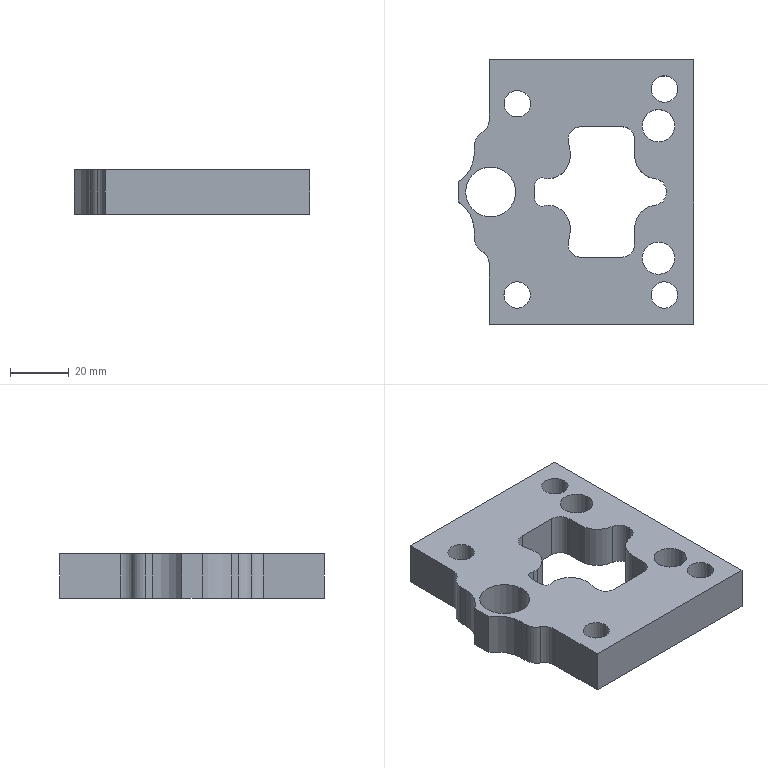Part | STEP file | 1 solid | 47 faces | box 80 x 90 x 15 mm | volume 69642 mm3 | cylinder 27 | plane 20 | commonest cylinder face diameters 8.28 x6 9 x4 10 x4 16.22 x4 5.28 x2 7.72 x2
STEP:
#1=CARTESIAN_POINT('',(347.5,22.5,-47.));
#2=VERTEX_POINT('',#1);
#3=CARTESIAN_POINT('',(342.,22.5,-47.));
#4=DIRECTION('',(0.,0.,1.));
#5=DIRECTION('',(1.,0.,0.));
#6=AXIS2_PLACEMENT_3D('',#3,#4,#5);
#7=CIRCLE('',#6,5.5);
#8=EDGE_CURVE('',#2,#2,#7,.T.);
#9=ORIENTED_EDGE('',*,*,#8,.T.);
#10=EDGE_LOOP('',(#9));
#11=FACE_BOUND('',#10,.T.);
#12=CARTESIAN_POINT('',(347.5,-22.5,-47.));
#13=VERTEX_POINT('',#12);
#14=CARTESIAN_POINT('',(342.,-22.5,-47.));
#15=DIRECTION('',(0.,0.,-1.));
#16=DIRECTION('',(1.,0.,0.));
#17=AXIS2_PLACEMENT_3D('',#14,#15,#16);
#18=CIRCLE('',#17,5.5);
#19=EDGE_CURVE('',#13,#13,#18,.T.);
#20=ORIENTED_EDGE('',*,*,#19,.F.);
#21=EDGE_LOOP('',(#20));
#22=FACE_BOUND('',#21,.T.);
#23=CARTESIAN_POINT('',(276.5,0.,-47.));
#24=VERTEX_POINT('',#23);
#25=CARTESIAN_POINT('',(285.,0.,-47.));
#26=DIRECTION('',(0.,0.,1.));
#27=DIRECTION('',(-1.,0.,0.));
#28=AXIS2_PLACEMENT_3D('',#25,#26,#27);
#29=CIRCLE('',#28,8.5);
#30=EDGE_CURVE('',#24,#24,#29,.T.);
#31=ORIENTED_EDGE('',*,*,#30,.T.);
#32=EDGE_LOOP('',(#31));
#33=FACE_BOUND('',#32,.T.);
#34=CARTESIAN_POINT('',(289.55,29.95,-47.));
#35=VERTEX_POINT('',#34);
#36=CARTESIAN_POINT('',(294.05,29.95,-47.));
#37=DIRECTION('',(0.,0.,1.));
#38=DIRECTION('',(-1.,0.,0.));
#39=AXIS2_PLACEMENT_3D('',#36,#37,#38);
#40=CIRCLE('',#39,4.5);
#41=EDGE_CURVE('',#35,#35,#40,.T.);
#42=ORIENTED_EDGE('',*,*,#41,.T.);
#43=EDGE_LOOP('',(#42));
#44=FACE_BOUND('',#43,.T.);
#45=CARTESIAN_POINT('',(339.55,34.95,-47.));
#46=VERTEX_POINT('',#45);
#47=CARTESIAN_POINT('',(344.05,34.95,-47.));
#48=DIRECTION('',(0.,0.,1.));
#49=DIRECTION('',(-1.,0.,0.));
#50=AXIS2_PLACEMENT_3D('',#47,#48,#49);
#51=CIRCLE('',#50,4.5);
#52=EDGE_CURVE('',#46,#46,#51,.T.);
#53=ORIENTED_EDGE('',*,*,#52,.T.);
#54=EDGE_LOOP('',(#53));
#55=FACE_BOUND('',#54,.T.);
#56=CARTESIAN_POINT('',(348.5,-35.,-47.));
#57=VERTEX_POINT('',#56);
#58=CARTESIAN_POINT('',(344.,-35.,-47.));
#59=DIRECTION('',(0.,0.,1.));
#60=DIRECTION('',(1.,0.,0.));
#61=AXIS2_PLACEMENT_3D('',#58,#59,#60);
#62=CIRCLE('',#61,4.5);
#63=EDGE_CURVE('',#57,#57,#62,.T.);
#64=ORIENTED_EDGE('',*,*,#63,.T.);
#65=EDGE_LOOP('',(#64));
#66=FACE_BOUND('',#65,.T.);
#67=CARTESIAN_POINT('',(298.5,-35.,-47.));
#68=VERTEX_POINT('',#67);
#69=CARTESIAN_POINT('',(294.,-35.,-47.));
#70=DIRECTION('',(0.,0.,1.));
#71=DIRECTION('',(1.,0.,0.));
#72=AXIS2_PLACEMENT_3D('',#69,#70,#71);
#73=CIRCLE('',#72,4.5);
#74=EDGE_CURVE('',#68,#68,#73,.T.);
#75=ORIENTED_EDGE('',*,*,#74,.T.);
#76=EDGE_LOOP('',(#75));
#77=FACE_BOUND('',#76,.T.);
#78=CARTESIAN_POINT('',(279.5,13.5,-47.));
#79=VERTEX_POINT('',#78);
#80=CARTESIAN_POINT('',(274.,3.413,-47.));
#81=VERTEX_POINT('',#80);
#82=CARTESIAN_POINT('',(267.5,13.5,-47.));
#83=DIRECTION('',(0.,0.,-1.));
#84=DIRECTION('',(-1.,0.,0.));
#85=AXIS2_PLACEMENT_3D('',#82,#83,#84);
#86=CIRCLE('',#85,12.);
#87=EDGE_CURVE('',#79,#81,#86,.T.);
#88=ORIENTED_EDGE('',*,*,#87,.F.);
#89=CARTESIAN_POINT('',(279.5,15.769,-47.));
#90=VERTEX_POINT('',#89);
#91=CARTESIAN_POINT('',(279.5,0.,-47.));
#92=DIRECTION('',(0.,-1.,0.));
#93=VECTOR('',#92,1.);
#94=LINE('',#91,#93);
#95=EDGE_CURVE('',#90,#79,#94,.T.);
#96=ORIENTED_EDGE('',*,*,#95,.F.);
#97=CARTESIAN_POINT('',(282.,20.099,-47.));
#98=VERTEX_POINT('',#97);
#99=CARTESIAN_POINT('',(284.5,15.769,-47.));
#100=DIRECTION('',(0.,0.,1.));
#101=DIRECTION('',(-1.,0.,0.));
#102=AXIS2_PLACEMENT_3D('',#99,#100,#101);
#103=CIRCLE('',#102,5.);
#104=EDGE_CURVE('',#98,#90,#103,.T.);
#105=ORIENTED_EDGE('',*,*,#104,.F.);
#106=CARTESIAN_POINT('',(284.5,24.429,-47.));
#107=VERTEX_POINT('',#106);
#108=CARTESIAN_POINT('',(279.5,24.429,-47.));
#109=DIRECTION('',(0.,0.,-1.));
#110=DIRECTION('',(-1.,0.,0.));
#111=AXIS2_PLACEMENT_3D('',#108,#109,#110);
#112=CIRCLE('',#111,5.);
#113=EDGE_CURVE('',#107,#98,#112,.T.);
#114=ORIENTED_EDGE('',*,*,#113,.F.);
#115=CARTESIAN_POINT('',(284.5,45.,-47.));
#116=VERTEX_POINT('',#115);
#117=CARTESIAN_POINT('',(284.5,0.,-47.));
#118=DIRECTION('',(0.,-1.,0.));
#119=VECTOR('',#118,1.);
#120=LINE('',#117,#119);
#121=EDGE_CURVE('',#116,#107,#120,.T.);
#122=ORIENTED_EDGE('',*,*,#121,.F.);
#123=CARTESIAN_POINT('',(354.,45.,-47.));
#124=VERTEX_POINT('',#123);
#125=CARTESIAN_POINT('',(323.,45.,-47.));
#126=DIRECTION('',(-1.,0.,0.));
#127=VECTOR('',#126,1.);
#128=LINE('',#125,#127);
#129=EDGE_CURVE('',#124,#116,#128,.T.);
#130=ORIENTED_EDGE('',*,*,#129,.F.);
#131=CARTESIAN_POINT('',(354.,-45.,-47.));
#132=VERTEX_POINT('',#131);
#133=CARTESIAN_POINT('',(354.,0.,-47.));
#134=DIRECTION('',(0.,1.,0.));
#135=VECTOR('',#134,1.);
#136=LINE('',#133,#135);
#137=EDGE_CURVE('',#132,#124,#136,.T.);
#138=ORIENTED_EDGE('',*,*,#137,.F.);
#139=CARTESIAN_POINT('',(284.5,-45.,-47.));
#140=VERTEX_POINT('',#139);
#141=CARTESIAN_POINT('',(323.,-45.,-47.));
#142=DIRECTION('',(1.,0.,0.));
#143=VECTOR('',#142,1.);
#144=LINE('',#141,#143);
#145=EDGE_CURVE('',#140,#132,#144,.T.);
#146=ORIENTED_EDGE('',*,*,#145,.F.);
#147=CARTESIAN_POINT('',(284.5,-24.429,-47.));
#148=VERTEX_POINT('',#147);
#149=CARTESIAN_POINT('',(284.5,0.,-47.));
#150=DIRECTION('',(0.,-1.,0.));
#151=VECTOR('',#150,1.);
#152=LINE('',#149,#151);
#153=EDGE_CURVE('',#148,#140,#152,.T.);
#154=ORIENTED_EDGE('',*,*,#153,.F.);
#155=CARTESIAN_POINT('',(282.,-20.099,-47.));
#156=VERTEX_POINT('',#155);
#157=CARTESIAN_POINT('',(279.5,-24.429,-47.));
#158=DIRECTION('',(0.,0.,1.));
#159=DIRECTION('',(-1.,0.,0.));
#160=AXIS2_PLACEMENT_3D('',#157,#158,#159);
#161=CIRCLE('',#160,5.);
#162=EDGE_CURVE('',#148,#156,#161,.T.);
#163=ORIENTED_EDGE('',*,*,#162,.T.);
#164=CARTESIAN_POINT('',(279.5,-15.769,-47.));
#165=VERTEX_POINT('',#164);
#166=CARTESIAN_POINT('',(284.5,-15.769,-47.));
#167=DIRECTION('',(0.,0.,-1.));
#168=DIRECTION('',(-1.,0.,0.));
#169=AXIS2_PLACEMENT_3D('',#166,#167,#168);
#170=CIRCLE('',#169,5.);
#171=EDGE_CURVE('',#156,#165,#170,.T.);
#172=ORIENTED_EDGE('',*,*,#171,.T.);
#173=CARTESIAN_POINT('',(279.5,-13.5,-47.));
#174=VERTEX_POINT('',#173);
#175=CARTESIAN_POINT('',(279.5,0.,-47.));
#176=DIRECTION('',(0.,-1.,0.));
#177=VECTOR('',#176,1.);
#178=LINE('',#175,#177);
#179=EDGE_CURVE('',#174,#165,#178,.T.);
#180=ORIENTED_EDGE('',*,*,#179,.F.);
#181=CARTESIAN_POINT('',(274.,-3.413,-47.));
#182=VERTEX_POINT('',#181);
#183=CARTESIAN_POINT('',(267.5,-13.5,-47.));
#184=DIRECTION('',(0.,0.,-1.));
#185=DIRECTION('',(-1.,0.,0.));
#186=AXIS2_PLACEMENT_3D('',#183,#184,#185);
#187=CIRCLE('',#186,12.);
#188=EDGE_CURVE('',#182,#174,#187,.T.);
#189=ORIENTED_EDGE('',*,*,#188,.F.);
#190=CARTESIAN_POINT('',(274.,0.,-47.));
#191=DIRECTION('',(0.,-1.,0.));
#192=VECTOR('',#191,1.);
#193=LINE('',#190,#192);
#194=EDGE_CURVE('',#81,#182,#193,.T.);
#195=ORIENTED_EDGE('',*,*,#194,.F.);
#196=EDGE_LOOP('',(#88,#96,#105,#114,#122,#130,#138,#146,#154,#163,#172,#180,#189,#195));
#197=FACE_BOUND('',#196,.T.);
#198=CARTESIAN_POINT('',(311.395,-17.285,-47.));
#199=VERTEX_POINT('',#198);
#200=CARTESIAN_POINT('',(315.473,-22.14,-47.));
#201=VERTEX_POINT('',#200);
#202=CARTESIAN_POINT('',(315.473,-18.,-47.));
#203=DIRECTION('',(0.,0.,1.));
#204=DIRECTION('',(-1.,0.,0.));
#205=AXIS2_PLACEMENT_3D('',#202,#203,#204);
#206=CIRCLE('',#205,4.14);
#207=EDGE_CURVE('',#199,#201,#206,.T.);
#208=ORIENTED_EDGE('',*,*,#207,.T.);
#209=CARTESIAN_POINT('',(329.75,-22.14,-47.));
#210=VERTEX_POINT('',#209);
#211=CARTESIAN_POINT('',(323.,-22.14,-47.));
#212=DIRECTION('',(-1.,0.,0.));
#213=VECTOR('',#212,1.);
#214=LINE('',#211,#213);
#215=EDGE_CURVE('',#210,#201,#214,.T.);
#216=ORIENTED_EDGE('',*,*,#215,.F.);
#217=CARTESIAN_POINT('',(333.89,-18.,-47.));
#218=VERTEX_POINT('',#217);
#219=CARTESIAN_POINT('',(329.75,-18.,-47.));
#220=DIRECTION('',(0.,0.,1.));
#221=DIRECTION('',(-1.,0.,0.));
#222=AXIS2_PLACEMENT_3D('',#219,#220,#221);
#223=CIRCLE('',#222,4.14);
#224=EDGE_CURVE('',#210,#218,#223,.T.);
#225=ORIENTED_EDGE('',*,*,#224,.T.);
#226=CARTESIAN_POINT('',(333.89,-12.5,-47.));
#227=VERTEX_POINT('',#226);
#228=CARTESIAN_POINT('',(333.89,0.,-47.));
#229=DIRECTION('',(0.,-1.,0.));
#230=VECTOR('',#229,1.);
#231=LINE('',#228,#230);
#232=EDGE_CURVE('',#227,#218,#231,.T.);
#233=ORIENTED_EDGE('',*,*,#232,.F.);
#234=CARTESIAN_POINT('',(341.007,-4.451,-47.));
#235=VERTEX_POINT('',#234);
#236=CARTESIAN_POINT('',(342.,-12.5,-47.));
#237=DIRECTION('',(0.,0.,1.));
#238=DIRECTION('',(-1.,0.,0.));
#239=AXIS2_PLACEMENT_3D('',#236,#237,#238);
#240=CIRCLE('',#239,8.11);
#241=EDGE_CURVE('',#235,#227,#240,.T.);
#242=ORIENTED_EDGE('',*,*,#241,.F.);
#243=CARTESIAN_POINT('',(344.64,-0.3422,-47.));
#244=VERTEX_POINT('',#243);
#245=CARTESIAN_POINT('',(340.5,-0.3422,-47.));
#246=DIRECTION('',(0.,0.,-1.));
#247=DIRECTION('',(-1.,0.,0.));
#248=AXIS2_PLACEMENT_3D('',#245,#246,#247);
#249=CIRCLE('',#248,4.14);
#250=EDGE_CURVE('',#244,#235,#249,.T.);
#251=ORIENTED_EDGE('',*,*,#250,.F.);
#252=CARTESIAN_POINT('',(344.64,0.3422,-47.));
#253=VERTEX_POINT('',#252);
#254=CARTESIAN_POINT('',(344.64,0.,-47.));
#255=DIRECTION('',(0.,-1.,0.));
#256=VECTOR('',#255,1.);
#257=LINE('',#254,#256);
#258=EDGE_CURVE('',#253,#244,#257,.T.);
#259=ORIENTED_EDGE('',*,*,#258,.F.);
#260=CARTESIAN_POINT('',(341.007,4.451,-47.));
#261=VERTEX_POINT('',#260);
#262=CARTESIAN_POINT('',(340.5,0.3422,-47.));
#263=DIRECTION('',(0.,0.,-1.));
#264=DIRECTION('',(-1.,0.,0.));
#265=AXIS2_PLACEMENT_3D('',#262,#263,#264);
#266=CIRCLE('',#265,4.14);
#267=EDGE_CURVE('',#261,#253,#266,.T.);
#268=ORIENTED_EDGE('',*,*,#267,.F.);
#269=CARTESIAN_POINT('',(333.89,12.5,-47.));
#270=VERTEX_POINT('',#269);
#271=CARTESIAN_POINT('',(342.,12.5,-47.));
#272=DIRECTION('',(0.,0.,1.));
#273=DIRECTION('',(-1.,0.,0.));
#274=AXIS2_PLACEMENT_3D('',#271,#272,#273);
#275=CIRCLE('',#274,8.11);
#276=EDGE_CURVE('',#270,#261,#275,.T.);
#277=ORIENTED_EDGE('',*,*,#276,.F.);
#278=CARTESIAN_POINT('',(333.89,18.,-47.));
#279=VERTEX_POINT('',#278);
#280=CARTESIAN_POINT('',(333.89,0.,-47.));
#281=DIRECTION('',(0.,-1.,0.));
#282=VECTOR('',#281,1.);
#283=LINE('',#280,#282);
#284=EDGE_CURVE('',#279,#270,#283,.T.);
#285=ORIENTED_EDGE('',*,*,#284,.F.);
#286=CARTESIAN_POINT('',(329.75,22.14,-47.));
#287=VERTEX_POINT('',#286);
#288=CARTESIAN_POINT('',(329.75,18.,-47.));
#289=DIRECTION('',(0.,0.,1.));
#290=DIRECTION('',(-1.,0.,0.));
#291=AXIS2_PLACEMENT_3D('',#288,#289,#290);
#292=CIRCLE('',#291,4.14);
#293=EDGE_CURVE('',#279,#287,#292,.T.);
#294=ORIENTED_EDGE('',*,*,#293,.T.);
#295=CARTESIAN_POINT('',(315.473,22.14,-47.));
#296=VERTEX_POINT('',#295);
#297=CARTESIAN_POINT('',(323.,22.14,-47.));
#298=DIRECTION('',(1.,0.,0.));
#299=VECTOR('',#298,1.);
#300=LINE('',#297,#299);
#301=EDGE_CURVE('',#296,#287,#300,.T.);
#302=ORIENTED_EDGE('',*,*,#301,.F.);
#303=CARTESIAN_POINT('',(311.395,17.285,-47.));
#304=VERTEX_POINT('',#303);
#305=CARTESIAN_POINT('',(315.473,18.,-47.));
#306=DIRECTION('',(0.,0.,1.));
#307=DIRECTION('',(-1.,0.,0.));
#308=AXIS2_PLACEMENT_3D('',#305,#306,#307);
#309=CIRCLE('',#308,4.14);
#310=EDGE_CURVE('',#296,#304,#309,.T.);
#311=ORIENTED_EDGE('',*,*,#310,.T.);
#312=CARTESIAN_POINT('',(311.988,13.9,-47.));
#313=VERTEX_POINT('',#312);
#314=CARTESIAN_POINT('',(314.681,-1.458,-47.));
#315=DIRECTION('',(-0.1727,0.985,0.));
#316=VECTOR('',#315,1.);
#317=LINE('',#314,#316);
#318=EDGE_CURVE('',#313,#304,#317,.T.);
#319=ORIENTED_EDGE('',*,*,#318,.F.);
#320=CARTESIAN_POINT('',(305.14,4.471,-47.));
#321=VERTEX_POINT('',#320);
#322=CARTESIAN_POINT('',(304.,12.5,-47.));
#323=DIRECTION('',(0.,0.,1.));
#324=DIRECTION('',(-1.,0.,0.));
#325=AXIS2_PLACEMENT_3D('',#322,#323,#324);
#326=CIRCLE('',#325,8.11);
#327=EDGE_CURVE('',#321,#313,#326,.T.);
#328=ORIENTED_EDGE('',*,*,#327,.F.);
#329=CARTESIAN_POINT('',(305.14,4.471,-47.));
#330=VERTEX_POINT('',#329);
#331=CARTESIAN_POINT('',(305.14,0.,-47.));
#332=DIRECTION('',(0.,-1.,0.));
#333=VECTOR('',#332,1.);
#334=LINE('',#331,#333);
#335=EDGE_CURVE('',#330,#321,#334,.T.);
#336=ORIENTED_EDGE('',*,*,#335,.F.);
#337=CARTESIAN_POINT('',(303.367,4.652,-47.));
#338=VERTEX_POINT('',#337);
#339=CARTESIAN_POINT('',(304.635,8.298,-47.));
#340=DIRECTION('',(0.,0.,1.));
#341=DIRECTION('',(-1.,0.,0.));
#342=AXIS2_PLACEMENT_3D('',#339,#340,#341);
#343=CIRCLE('',#342,3.86);
#344=EDGE_CURVE('',#338,#330,#343,.T.);
#345=ORIENTED_EDGE('',*,*,#344,.F.);
#346=CARTESIAN_POINT('',(299.86,2.158,-47.));
#347=VERTEX_POINT('',#346);
#348=CARTESIAN_POINT('',(302.5,2.158,-47.));
#349=DIRECTION('',(0.,0.,-1.));
#350=DIRECTION('',(-1.,0.,0.));
#351=AXIS2_PLACEMENT_3D('',#348,#349,#350);
#352=CIRCLE('',#351,2.64);
#353=EDGE_CURVE('',#347,#338,#352,.T.);
#354=ORIENTED_EDGE('',*,*,#353,.F.);
#355=CARTESIAN_POINT('',(299.86,-2.158,-47.));
#356=VERTEX_POINT('',#355);
#357=CARTESIAN_POINT('',(299.86,0.,-47.));
#358=DIRECTION('',(0.,1.,0.));
#359=VECTOR('',#358,1.);
#360=LINE('',#357,#359);
#361=EDGE_CURVE('',#356,#347,#360,.T.);
#362=ORIENTED_EDGE('',*,*,#361,.F.);
#363=CARTESIAN_POINT('',(303.367,-4.652,-47.));
#364=VERTEX_POINT('',#363);
#365=CARTESIAN_POINT('',(302.5,-2.158,-47.));
#366=DIRECTION('',(0.,0.,-1.));
#367=DIRECTION('',(-1.,0.,0.));
#368=AXIS2_PLACEMENT_3D('',#365,#366,#367);
#369=CIRCLE('',#368,2.64);
#370=EDGE_CURVE('',#364,#356,#369,.T.);
#371=ORIENTED_EDGE('',*,*,#370,.F.);
#372=CARTESIAN_POINT('',(305.14,-4.471,-47.));
#373=VERTEX_POINT('',#372);
#374=CARTESIAN_POINT('',(304.635,-8.298,-47.));
#375=DIRECTION('',(0.,0.,1.));
#376=DIRECTION('',(-1.,0.,0.));
#377=AXIS2_PLACEMENT_3D('',#374,#375,#376);
#378=CIRCLE('',#377,3.86);
#379=EDGE_CURVE('',#373,#364,#378,.T.);
#380=ORIENTED_EDGE('',*,*,#379,.F.);
#381=CARTESIAN_POINT('',(305.14,-4.471,-47.));
#382=VERTEX_POINT('',#381);
#383=CARTESIAN_POINT('',(305.14,0.,-47.));
#384=DIRECTION('',(0.,-1.,0.));
#385=VECTOR('',#384,1.);
#386=LINE('',#383,#385);
#387=EDGE_CURVE('',#382,#373,#386,.T.);
#388=ORIENTED_EDGE('',*,*,#387,.F.);
#389=CARTESIAN_POINT('',(311.988,-13.9,-47.));
#390=VERTEX_POINT('',#389);
#391=CARTESIAN_POINT('',(304.,-12.5,-47.));
#392=DIRECTION('',(0.,0.,1.));
#393=DIRECTION('',(-1.,0.,0.));
#394=AXIS2_PLACEMENT_3D('',#391,#392,#393);
#395=CIRCLE('',#394,8.11);
#396=EDGE_CURVE('',#390,#382,#395,.T.);
#397=ORIENTED_EDGE('',*,*,#396,.F.);
#398=CARTESIAN_POINT('',(314.681,1.458,-47.));
#399=DIRECTION('',(0.1727,0.985,0.));
#400=VECTOR('',#399,1.);
#401=LINE('',#398,#400);
#402=EDGE_CURVE('',#199,#390,#401,.T.);
#403=ORIENTED_EDGE('',*,*,#402,.F.);
#404=EDGE_LOOP('',(#208,#216,#225,#233,#242,#251,#259,#268,#277,#285,#294,#302,#311,#319,#328,#336,#345,#354,#362,#371,#380,#388,#397,#403));
#405=FACE_BOUND('',#404,.T.);
#406=CARTESIAN_POINT('',(323.,0.,-47.));
#407=DIRECTION('',(0.,0.,-1.));
#408=DIRECTION('',(-1.,0.,0.));
#409=AXIS2_PLACEMENT_3D('',#406,#407,#408);
#410=PLANE('',#409);
#411=ADVANCED_FACE('',(#11,#22,#33,#44,#55,#66,#77,#197,#405),#410,.T.);
#412=CARTESIAN_POINT('',(274.,3.413,-32.));
#413=VERTEX_POINT('',#412);
#414=CARTESIAN_POINT('',(274.,-3.413,-32.));
#415=VERTEX_POINT('',#414);
#416=CARTESIAN_POINT('',(274.,0.,-32.));
#417=DIRECTION('',(0.,-1.,0.));
#418=VECTOR('',#417,1.);
#419=LINE('',#416,#418);
#420=EDGE_CURVE('',#413,#415,#419,.T.);
#421=ORIENTED_EDGE('',*,*,#420,.F.);
#422=CARTESIAN_POINT('',(274.,3.413,-53.));
#423=DIRECTION('',(0.,0.,-1.));
#424=VECTOR('',#423,1.);
#425=LINE('',#422,#424);
#426=EDGE_CURVE('',#413,#81,#425,.T.);
#427=ORIENTED_EDGE('',*,*,#426,.T.);
#428=ORIENTED_EDGE('',*,*,#194,.T.);
#429=CARTESIAN_POINT('',(274.,-3.413,-83.));
#430=DIRECTION('',(0.,0.,1.));
#431=VECTOR('',#430,1.);
#432=LINE('',#429,#431);
#433=EDGE_CURVE('',#182,#415,#432,.T.);
#434=ORIENTED_EDGE('',*,*,#433,.T.);
#435=EDGE_LOOP('',(#421,#427,#428,#434));
#436=FACE_OUTER_BOUND('',#435,.T.);
#437=CARTESIAN_POINT('',(274.,0.,-17.));
#438=DIRECTION('',(1.,0.,0.));
#439=DIRECTION('',(0.,0.,-1.));
#440=AXIS2_PLACEMENT_3D('',#437,#438,#439);
#441=PLANE('',#440);
#442=ADVANCED_FACE('',(#436),#441,.F.);
#443=ORIENTED_EDGE('',*,*,#129,.T.);
#444=CARTESIAN_POINT('',(284.5,45.,-32.));
#445=VERTEX_POINT('',#444);
#446=CARTESIAN_POINT('',(284.5,45.,-53.));
#447=DIRECTION('',(0.,0.,1.));
#448=VECTOR('',#447,1.);
#449=LINE('',#446,#448);
#450=EDGE_CURVE('',#116,#445,#449,.T.);
#451=ORIENTED_EDGE('',*,*,#450,.T.);
#452=CARTESIAN_POINT('',(354.,45.,-32.));
#453=VERTEX_POINT('',#452);
#454=CARTESIAN_POINT('',(323.,45.,-32.));
#455=DIRECTION('',(-1.,0.,0.));
#456=VECTOR('',#455,1.);
#457=LINE('',#454,#456);
#458=EDGE_CURVE('',#453,#445,#457,.T.);
#459=ORIENTED_EDGE('',*,*,#458,.F.);
#460=CARTESIAN_POINT('',(354.,45.,-32.));
#461=DIRECTION('',(0.,0.,-1.));
#462=VECTOR('',#461,1.);
#463=LINE('',#460,#462);
#464=EDGE_CURVE('',#453,#124,#463,.T.);
#465=ORIENTED_EDGE('',*,*,#464,.T.);
#466=EDGE_LOOP('',(#443,#451,#459,#465));
#467=FACE_OUTER_BOUND('',#466,.T.);
#468=CARTESIAN_POINT('',(323.,45.,-32.));
#469=DIRECTION('',(0.,-1.,0.));
#470=DIRECTION('',(-1.,0.,0.));
#471=AXIS2_PLACEMENT_3D('',#468,#469,#470);
#472=PLANE('',#471);
#473=ADVANCED_FACE('',(#467),#472,.F.);
#474=CARTESIAN_POINT('',(329.75,-22.14,-32.));
#475=VERTEX_POINT('',#474);
#476=CARTESIAN_POINT('',(315.473,-22.14,-32.));
#477=VERTEX_POINT('',#476);
#478=CARTESIAN_POINT('',(323.,-22.14,-32.));
#479=DIRECTION('',(-1.,0.,0.));
#480=VECTOR('',#479,1.);
#481=LINE('',#478,#480);
#482=EDGE_CURVE('',#475,#477,#481,.T.);
#483=ORIENTED_EDGE('',*,*,#482,.F.);
#484=CARTESIAN_POINT('',(329.75,-22.14,-32.));
#485=DIRECTION('',(0.,0.,-1.));
#486=VECTOR('',#485,1.);
#487=LINE('',#484,#486);
#488=EDGE_CURVE('',#475,#210,#487,.T.);
#489=ORIENTED_EDGE('',*,*,#488,.T.);
#490=ORIENTED_EDGE('',*,*,#215,.T.);
#491=CARTESIAN_POINT('',(315.473,-22.14,-32.));
#492=DIRECTION('',(0.,0.,-1.));
#493=VECTOR('',#492,1.);
#494=LINE('',#491,#493);
#495=EDGE_CURVE('',#477,#201,#494,.T.);
#496=ORIENTED_EDGE('',*,*,#495,.F.);
#497=EDGE_LOOP('',(#483,#489,#490,#496));
#498=FACE_OUTER_BOUND('',#497,.T.);
#499=CARTESIAN_POINT('',(323.,-22.14,-32.));
#500=DIRECTION('',(0.,-1.,0.));
#501=DIRECTION('',(-1.,0.,0.));
#502=AXIS2_PLACEMENT_3D('',#499,#500,#501);
#503=PLANE('',#502);
#504=ADVANCED_FACE('',(#498),#503,.F.);
#505=ORIENTED_EDGE('',*,*,#488,.F.);
#506=CARTESIAN_POINT('',(333.89,-18.,-32.));
#507=VERTEX_POINT('',#506);
#508=CARTESIAN_POINT('',(329.75,-18.,-32.));
#509=DIRECTION('',(0.,0.,1.));
#510=DIRECTION('',(-1.,0.,0.));
#511=AXIS2_PLACEMENT_3D('',#508,#509,#510);
#512=CIRCLE('',#511,4.14);
#513=EDGE_CURVE('',#475,#507,#512,.T.);
#514=ORIENTED_EDGE('',*,*,#513,.T.);
#515=CARTESIAN_POINT('',(333.89,-18.,-32.));
#516=DIRECTION('',(0.,0.,-1.));
#517=VECTOR('',#516,1.);
#518=LINE('',#515,#517);
#519=EDGE_CURVE('',#507,#218,#518,.T.);
#520=ORIENTED_EDGE('',*,*,#519,.T.);
#521=ORIENTED_EDGE('',*,*,#224,.F.);
#522=EDGE_LOOP('',(#505,#514,#520,#521));
#523=FACE_OUTER_BOUND('',#522,.T.);
#524=CARTESIAN_POINT('',(329.75,-18.,-32.));
#525=DIRECTION('',(0.,0.,-1.));
#526=DIRECTION('',(-1.,0.,0.));
#527=AXIS2_PLACEMENT_3D('',#524,#525,#526);
#528=CYLINDRICAL_SURFACE('',#527,4.14);
#529=ADVANCED_FACE('',(#523),#528,.F.);
#530=ORIENTED_EDGE('',*,*,#519,.F.);
#531=CARTESIAN_POINT('',(333.89,-12.5,-32.));
#532=VERTEX_POINT('',#531);
#533=CARTESIAN_POINT('',(333.89,0.,-32.));
#534=DIRECTION('',(0.,-1.,0.));
#535=VECTOR('',#534,1.);
#536=LINE('',#533,#535);
#537=EDGE_CURVE('',#532,#507,#536,.T.);
#538=ORIENTED_EDGE('',*,*,#537,.F.);
#539=CARTESIAN_POINT('',(333.89,-12.5,-32.));
#540=DIRECTION('',(0.,0.,-1.));
#541=VECTOR('',#540,1.);
#542=LINE('',#539,#541);
#543=EDGE_CURVE('',#532,#227,#542,.T.);
#544=ORIENTED_EDGE('',*,*,#543,.T.);
#545=ORIENTED_EDGE('',*,*,#232,.T.);
#546=EDGE_LOOP('',(#530,#538,#544,#545));
#547=FACE_OUTER_BOUND('',#546,.T.);
#548=CARTESIAN_POINT('',(333.89,0.,-32.));
#549=DIRECTION('',(-1.,0.,0.));
#550=DIRECTION('',(0.,1.,0.));
#551=AXIS2_PLACEMENT_3D('',#548,#549,#550);
#552=PLANE('',#551);
#553=ADVANCED_FACE('',(#547),#552,.T.);
#554=ORIENTED_EDGE('',*,*,#543,.F.);
#555=CARTESIAN_POINT('',(341.007,-4.451,-32.));
#556=VERTEX_POINT('',#555);
#557=CARTESIAN_POINT('',(342.,-12.5,-32.));
#558=DIRECTION('',(0.,0.,1.));
#559=DIRECTION('',(-1.,0.,0.));
#560=AXIS2_PLACEMENT_3D('',#557,#558,#559);
#561=CIRCLE('',#560,8.11);
#562=EDGE_CURVE('',#556,#532,#561,.T.);
#563=ORIENTED_EDGE('',*,*,#562,.F.);
#564=CARTESIAN_POINT('',(341.007,-4.451,-32.));
#565=DIRECTION('',(0.,0.,-1.));
#566=VECTOR('',#565,1.);
#567=LINE('',#564,#566);
#568=EDGE_CURVE('',#556,#235,#567,.T.);
#569=ORIENTED_EDGE('',*,*,#568,.T.);
#570=ORIENTED_EDGE('',*,*,#241,.T.);
#571=EDGE_LOOP('',(#554,#563,#569,#570));
#572=FACE_OUTER_BOUND('',#571,.T.);
#573=CARTESIAN_POINT('',(342.,-12.5,-32.));
#574=DIRECTION('',(0.,0.,-1.));
#575=DIRECTION('',(-1.,0.,0.));
#576=AXIS2_PLACEMENT_3D('',#573,#574,#575);
#577=CYLINDRICAL_SURFACE('',#576,8.11);
#578=ADVANCED_FACE('',(#572),#577,.T.);
#579=ORIENTED_EDGE('',*,*,#568,.F.);
#580=CARTESIAN_POINT('',(344.64,-0.3422,-32.));
#581=VERTEX_POINT('',#580);
#582=CARTESIAN_POINT('',(340.5,-0.3422,-32.));
#583=DIRECTION('',(0.,0.,-1.));
#584=DIRECTION('',(-1.,0.,0.));
#585=AXIS2_PLACEMENT_3D('',#582,#583,#584);
#586=CIRCLE('',#585,4.14);
#587=EDGE_CURVE('',#581,#556,#586,.T.);
#588=ORIENTED_EDGE('',*,*,#587,.F.);
#589=CARTESIAN_POINT('',(344.64,-0.3422,-32.));
#590=DIRECTION('',(0.,0.,-1.));
#591=VECTOR('',#590,1.);
#592=LINE('',#589,#591);
#593=EDGE_CURVE('',#581,#244,#592,.T.);
#594=ORIENTED_EDGE('',*,*,#593,.T.);
#595=ORIENTED_EDGE('',*,*,#250,.T.);
#596=EDGE_LOOP('',(#579,#588,#594,#595));
#597=FACE_OUTER_BOUND('',#596,.T.);
#598=CARTESIAN_POINT('',(340.5,-0.3422,-32.));
#599=DIRECTION('',(0.,0.,-1.));
#600=DIRECTION('',(-1.,0.,0.));
#601=AXIS2_PLACEMENT_3D('',#598,#599,#600);
#602=CYLINDRICAL_SURFACE('',#601,4.14);
#603=ADVANCED_FACE('',(#597),#602,.F.);
#604=ORIENTED_EDGE('',*,*,#593,.F.);
#605=CARTESIAN_POINT('',(344.64,0.3422,-32.));
#606=VERTEX_POINT('',#605);
#607=CARTESIAN_POINT('',(344.64,0.,-32.));
#608=DIRECTION('',(0.,-1.,0.));
#609=VECTOR('',#608,1.);
#610=LINE('',#607,#609);
#611=EDGE_CURVE('',#606,#581,#610,.T.);
#612=ORIENTED_EDGE('',*,*,#611,.F.);
#613=CARTESIAN_POINT('',(344.64,0.3422,-32.));
#614=DIRECTION('',(0.,0.,-1.));
#615=VECTOR('',#614,1.);
#616=LINE('',#613,#615);
#617=EDGE_CURVE('',#606,#253,#616,.T.);
#618=ORIENTED_EDGE('',*,*,#617,.T.);
#619=ORIENTED_EDGE('',*,*,#258,.T.);
#620=EDGE_LOOP('',(#604,#612,#618,#619));
#621=FACE_OUTER_BOUND('',#620,.T.);
#622=CARTESIAN_POINT('',(344.64,0.,-32.));
#623=DIRECTION('',(-1.,0.,0.));
#624=DIRECTION('',(0.,1.,0.));
#625=AXIS2_PLACEMENT_3D('',#622,#623,#624);
#626=PLANE('',#625);
#627=ADVANCED_FACE('',(#621),#626,.T.);
#628=ORIENTED_EDGE('',*,*,#617,.F.);
#629=CARTESIAN_POINT('',(341.007,4.451,-32.));
#630=VERTEX_POINT('',#629);
#631=CARTESIAN_POINT('',(340.5,0.3422,-32.));
#632=DIRECTION('',(0.,0.,-1.));
#633=DIRECTION('',(-1.,0.,0.));
#634=AXIS2_PLACEMENT_3D('',#631,#632,#633);
#635=CIRCLE('',#634,4.14);
#636=EDGE_CURVE('',#630,#606,#635,.T.);
#637=ORIENTED_EDGE('',*,*,#636,.F.);
#638=CARTESIAN_POINT('',(341.007,4.451,-32.));
#639=DIRECTION('',(0.,0.,-1.));
#640=VECTOR('',#639,1.);
#641=LINE('',#638,#640);
#642=EDGE_CURVE('',#630,#261,#641,.T.);
#643=ORIENTED_EDGE('',*,*,#642,.T.);
#644=ORIENTED_EDGE('',*,*,#267,.T.);
#645=EDGE_LOOP('',(#628,#637,#643,#644));
#646=FACE_OUTER_BOUND('',#645,.T.);
#647=CARTESIAN_POINT('',(340.5,0.3422,-32.));
#648=DIRECTION('',(0.,0.,-1.));
#649=DIRECTION('',(-1.,0.,0.));
#650=AXIS2_PLACEMENT_3D('',#647,#648,#649);
#651=CYLINDRICAL_SURFACE('',#650,4.14);
#652=ADVANCED_FACE('',(#646),#651,.F.);
#653=ORIENTED_EDGE('',*,*,#642,.F.);
#654=CARTESIAN_POINT('',(333.89,12.5,-32.));
#655=VERTEX_POINT('',#654);
#656=CARTESIAN_POINT('',(342.,12.5,-32.));
#657=DIRECTION('',(0.,0.,1.));
#658=DIRECTION('',(-1.,0.,0.));
#659=AXIS2_PLACEMENT_3D('',#656,#657,#658);
#660=CIRCLE('',#659,8.11);
#661=EDGE_CURVE('',#655,#630,#660,.T.);
#662=ORIENTED_EDGE('',*,*,#661,.F.);
#663=CARTESIAN_POINT('',(333.89,12.5,-32.));
#664=DIRECTION('',(0.,0.,-1.));
#665=VECTOR('',#664,1.);
#666=LINE('',#663,#665);
#667=EDGE_CURVE('',#655,#270,#666,.T.);
#668=ORIENTED_EDGE('',*,*,#667,.T.);
#669=ORIENTED_EDGE('',*,*,#276,.T.);
#670=EDGE_LOOP('',(#653,#662,#668,#669));
#671=FACE_OUTER_BOUND('',#670,.T.);
#672=CARTESIAN_POINT('',(342.,12.5,-32.));
#673=DIRECTION('',(0.,0.,-1.));
#674=DIRECTION('',(-1.,0.,0.));
#675=AXIS2_PLACEMENT_3D('',#672,#673,#674);
#676=CYLINDRICAL_SURFACE('',#675,8.11);
#677=ADVANCED_FACE('',(#671),#676,.T.);
#678=ORIENTED_EDGE('',*,*,#667,.F.);
#679=CARTESIAN_POINT('',(333.89,18.,-32.));
#680=VERTEX_POINT('',#679);
#681=CARTESIAN_POINT('',(333.89,0.,-32.));
#682=DIRECTION('',(0.,-1.,0.));
#683=VECTOR('',#682,1.);
#684=LINE('',#681,#683);
#685=EDGE_CURVE('',#680,#655,#684,.T.);
#686=ORIENTED_EDGE('',*,*,#685,.F.);
#687=CARTESIAN_POINT('',(333.89,18.,-32.));
#688=DIRECTION('',(0.,0.,-1.));
#689=VECTOR('',#688,1.);
#690=LINE('',#687,#689);
#691=EDGE_CURVE('',#680,#279,#690,.T.);
#692=ORIENTED_EDGE('',*,*,#691,.T.);
#693=ORIENTED_EDGE('',*,*,#284,.T.);
#694=EDGE_LOOP('',(#678,#686,#692,#693));
#695=FACE_OUTER_BOUND('',#694,.T.);
#696=CARTESIAN_POINT('',(333.89,0.,-32.));
#697=DIRECTION('',(1.,0.,0.));
#698=DIRECTION('',(0.,-1.,0.));
#699=AXIS2_PLACEMENT_3D('',#696,#697,#698);
#700=PLANE('',#699);
#701=ADVANCED_FACE('',(#695),#700,.F.);
#702=ORIENTED_EDGE('',*,*,#691,.F.);
#703=CARTESIAN_POINT('',(329.75,22.14,-32.));
#704=VERTEX_POINT('',#703);
#705=CARTESIAN_POINT('',(329.75,18.,-32.));
#706=DIRECTION('',(0.,0.,1.));
#707=DIRECTION('',(-1.,0.,0.));
#708=AXIS2_PLACEMENT_3D('',#705,#706,#707);
#709=CIRCLE('',#708,4.14);
#710=EDGE_CURVE('',#680,#704,#709,.T.);
#711=ORIENTED_EDGE('',*,*,#710,.T.);
#712=CARTESIAN_POINT('',(329.75,22.14,-32.));
#713=DIRECTION('',(0.,0.,-1.));
#714=VECTOR('',#713,1.);
#715=LINE('',#712,#714);
#716=EDGE_CURVE('',#704,#287,#715,.T.);
#717=ORIENTED_EDGE('',*,*,#716,.T.);
#718=ORIENTED_EDGE('',*,*,#293,.F.);
#719=EDGE_LOOP('',(#702,#711,#717,#718));
#720=FACE_OUTER_BOUND('',#719,.T.);
#721=CARTESIAN_POINT('',(329.75,18.,-32.));
#722=DIRECTION('',(0.,0.,-1.));
#723=DIRECTION('',(-1.,0.,0.));
#724=AXIS2_PLACEMENT_3D('',#721,#722,#723);
#725=CYLINDRICAL_SURFACE('',#724,4.14);
#726=ADVANCED_FACE('',(#720),#725,.F.);
#727=ORIENTED_EDGE('',*,*,#716,.F.);
#728=CARTESIAN_POINT('',(315.473,22.14,-32.));
#729=VERTEX_POINT('',#728);
#730=CARTESIAN_POINT('',(323.,22.14,-32.));
#731=DIRECTION('',(1.,0.,0.));
#732=VECTOR('',#731,1.);
#733=LINE('',#730,#732);
#734=EDGE_CURVE('',#729,#704,#733,.T.);
#735=ORIENTED_EDGE('',*,*,#734,.F.);
#736=CARTESIAN_POINT('',(315.473,22.14,-32.));
#737=DIRECTION('',(0.,0.,-1.));
#738=VECTOR('',#737,1.);
#739=LINE('',#736,#738);
#740=EDGE_CURVE('',#729,#296,#739,.T.);
#741=ORIENTED_EDGE('',*,*,#740,.T.);
#742=ORIENTED_EDGE('',*,*,#301,.T.);
#743=EDGE_LOOP('',(#727,#735,#741,#742));
#744=FACE_OUTER_BOUND('',#743,.T.);
#745=CARTESIAN_POINT('',(323.,22.14,-32.));
#746=DIRECTION('',(0.,1.,0.));
#747=DIRECTION('',(1.,0.,0.));
#748=AXIS2_PLACEMENT_3D('',#745,#746,#747);
#749=PLANE('',#748);
#750=ADVANCED_FACE('',(#744),#749,.F.);
#751=ORIENTED_EDGE('',*,*,#740,.F.);
#752=CARTESIAN_POINT('',(311.395,17.285,-32.));
#753=VERTEX_POINT('',#752);
#754=CARTESIAN_POINT('',(315.473,18.,-32.));
#755=DIRECTION('',(0.,0.,1.));
#756=DIRECTION('',(-1.,0.,0.));
#757=AXIS2_PLACEMENT_3D('',#754,#755,#756);
#758=CIRCLE('',#757,4.14);
#759=EDGE_CURVE('',#729,#753,#758,.T.);
#760=ORIENTED_EDGE('',*,*,#759,.T.);
#761=CARTESIAN_POINT('',(311.395,17.285,-32.));
#762=DIRECTION('',(0.,0.,-1.));
#763=VECTOR('',#762,1.);
#764=LINE('',#761,#763);
#765=EDGE_CURVE('',#753,#304,#764,.T.);
#766=ORIENTED_EDGE('',*,*,#765,.T.);
#767=ORIENTED_EDGE('',*,*,#310,.F.);
#768=EDGE_LOOP('',(#751,#760,#766,#767));
#769=FACE_OUTER_BOUND('',#768,.T.);
#770=CARTESIAN_POINT('',(315.473,18.,-32.));
#771=DIRECTION('',(0.,0.,-1.));
#772=DIRECTION('',(-1.,0.,0.));
#773=AXIS2_PLACEMENT_3D('',#770,#771,#772);
#774=CYLINDRICAL_SURFACE('',#773,4.14);
#775=ADVANCED_FACE('',(#769),#774,.F.);
#776=ORIENTED_EDGE('',*,*,#765,.F.);
#777=CARTESIAN_POINT('',(311.988,13.9,-32.));
#778=VERTEX_POINT('',#777);
#779=CARTESIAN_POINT('',(314.681,-1.458,-32.));
#780=DIRECTION('',(-0.1727,0.985,0.));
#781=VECTOR('',#780,1.);
#782=LINE('',#779,#781);
#783=EDGE_CURVE('',#778,#753,#782,.T.);
#784=ORIENTED_EDGE('',*,*,#783,.F.);
#785=CARTESIAN_POINT('',(311.988,13.9,-32.));
#786=DIRECTION('',(0.,0.,-1.));
#787=VECTOR('',#786,1.);
#788=LINE('',#785,#787);
#789=EDGE_CURVE('',#778,#313,#788,.T.);
#790=ORIENTED_EDGE('',*,*,#789,.T.);
#791=ORIENTED_EDGE('',*,*,#318,.T.);
#792=EDGE_LOOP('',(#776,#784,#790,#791));
#793=FACE_OUTER_BOUND('',#792,.T.);
#794=CARTESIAN_POINT('',(314.681,-1.458,-32.));
#795=DIRECTION('',(-0.985,-0.1727,0.));
#796=DIRECTION('',(-0.1727,0.985,0.));
#797=AXIS2_PLACEMENT_3D('',#794,#795,#796);
#798=PLANE('',#797);
#799=ADVANCED_FACE('',(#793),#798,.F.);
#800=ORIENTED_EDGE('',*,*,#789,.F.);
#801=CARTESIAN_POINT('',(305.14,4.471,-32.));
#802=VERTEX_POINT('',#801);
#803=CARTESIAN_POINT('',(304.,12.5,-32.));
#804=DIRECTION('',(0.,0.,1.));
#805=DIRECTION('',(-1.,0.,0.));
#806=AXIS2_PLACEMENT_3D('',#803,#804,#805);
#807=CIRCLE('',#806,8.11);
#808=EDGE_CURVE('',#802,#778,#807,.T.);
#809=ORIENTED_EDGE('',*,*,#808,.F.);
#810=CARTESIAN_POINT('',(305.14,4.471,-32.));
#811=DIRECTION('',(0.,0.,-1.));
#812=VECTOR('',#811,1.);
#813=LINE('',#810,#812);
#814=EDGE_CURVE('',#802,#321,#813,.T.);
#815=ORIENTED_EDGE('',*,*,#814,.T.);
#816=ORIENTED_EDGE('',*,*,#327,.T.);
#817=EDGE_LOOP('',(#800,#809,#815,#816));
#818=FACE_OUTER_BOUND('',#817,.T.);
#819=CARTESIAN_POINT('',(304.,12.5,-32.));
#820=DIRECTION('',(0.,0.,-1.));
#821=DIRECTION('',(-1.,0.,0.));
#822=AXIS2_PLACEMENT_3D('',#819,#820,#821);
#823=CYLINDRICAL_SURFACE('',#822,8.11);
#824=ADVANCED_FACE('',(#818),#823,.T.);
#825=ORIENTED_EDGE('',*,*,#814,.F.);
#826=CARTESIAN_POINT('',(305.14,4.471,-32.));
#827=VERTEX_POINT('',#826);
#828=CARTESIAN_POINT('',(305.14,0.,-32.));
#829=DIRECTION('',(0.,-1.,0.));
#830=VECTOR('',#829,1.);
#831=LINE('',#828,#830);
#832=EDGE_CURVE('',#827,#802,#831,.T.);
#833=ORIENTED_EDGE('',*,*,#832,.F.);
#834=CARTESIAN_POINT('',(305.14,4.471,-32.));
#835=DIRECTION('',(0.,0.,-1.));
#836=VECTOR('',#835,1.);
#837=LINE('',#834,#836);
#838=EDGE_CURVE('',#827,#330,#837,.T.);
#839=ORIENTED_EDGE('',*,*,#838,.T.);
#840=ORIENTED_EDGE('',*,*,#335,.T.);
#841=EDGE_LOOP('',(#825,#833,#839,#840));
#842=FACE_OUTER_BOUND('',#841,.T.);
#843=CARTESIAN_POINT('',(305.14,0.,-32.));
#844=DIRECTION('',(-1.,0.,0.));
#845=DIRECTION('',(0.,1.,0.));
#846=AXIS2_PLACEMENT_3D('',#843,#844,#845);
#847=PLANE('',#846);
#848=ADVANCED_FACE('',(#842),#847,.T.);
#849=ORIENTED_EDGE('',*,*,#838,.F.);
#850=CARTESIAN_POINT('',(303.367,4.652,-32.));
#851=VERTEX_POINT('',#850);
#852=CARTESIAN_POINT('',(304.635,8.298,-32.));
#853=DIRECTION('',(0.,0.,1.));
#854=DIRECTION('',(-1.,0.,0.));
#855=AXIS2_PLACEMENT_3D('',#852,#853,#854);
#856=CIRCLE('',#855,3.86);
#857=EDGE_CURVE('',#851,#827,#856,.T.);
#858=ORIENTED_EDGE('',*,*,#857,.F.);
#859=CARTESIAN_POINT('',(303.367,4.652,-32.));
#860=DIRECTION('',(0.,0.,-1.));
#861=VECTOR('',#860,1.);
#862=LINE('',#859,#861);
#863=EDGE_CURVE('',#851,#338,#862,.T.);
#864=ORIENTED_EDGE('',*,*,#863,.T.);
#865=ORIENTED_EDGE('',*,*,#344,.T.);
#866=EDGE_LOOP('',(#849,#858,#864,#865));
#867=FACE_OUTER_BOUND('',#866,.T.);
#868=CARTESIAN_POINT('',(304.635,8.298,-32.));
#869=DIRECTION('',(0.,0.,-1.));
#870=DIRECTION('',(-1.,0.,0.));
#871=AXIS2_PLACEMENT_3D('',#868,#869,#870);
#872=CYLINDRICAL_SURFACE('',#871,3.86);
#873=ADVANCED_FACE('',(#867),#872,.T.);
#874=ORIENTED_EDGE('',*,*,#863,.F.);
#875=CARTESIAN_POINT('',(299.86,2.158,-32.));
#876=VERTEX_POINT('',#875);
#877=CARTESIAN_POINT('',(302.5,2.158,-32.));
#878=DIRECTION('',(0.,0.,-1.));
#879=DIRECTION('',(-1.,0.,0.));
#880=AXIS2_PLACEMENT_3D('',#877,#878,#879);
#881=CIRCLE('',#880,2.64);
#882=EDGE_CURVE('',#876,#851,#881,.T.);
#883=ORIENTED_EDGE('',*,*,#882,.F.);
#884=CARTESIAN_POINT('',(299.86,2.158,-32.));
#885=DIRECTION('',(0.,0.,-1.));
#886=VECTOR('',#885,1.);
#887=LINE('',#884,#886);
#888=EDGE_CURVE('',#876,#347,#887,.T.);
#889=ORIENTED_EDGE('',*,*,#888,.T.);
#890=ORIENTED_EDGE('',*,*,#353,.T.);
#891=EDGE_LOOP('',(#874,#883,#889,#890));
#892=FACE_OUTER_BOUND('',#891,.T.);
#893=CARTESIAN_POINT('',(302.5,2.158,-32.));
#894=DIRECTION('',(0.,0.,-1.));
#895=DIRECTION('',(-1.,0.,0.));
#896=AXIS2_PLACEMENT_3D('',#893,#894,#895);
#897=CYLINDRICAL_SURFACE('',#896,2.64);
#898=ADVANCED_FACE('',(#892),#897,.F.);
#899=ORIENTED_EDGE('',*,*,#888,.F.);
#900=CARTESIAN_POINT('',(299.86,-2.158,-32.));
#901=VERTEX_POINT('',#900);
#902=CARTESIAN_POINT('',(299.86,0.,-32.));
#903=DIRECTION('',(0.,1.,0.));
#904=VECTOR('',#903,1.);
#905=LINE('',#902,#904);
#906=EDGE_CURVE('',#901,#876,#905,.T.);
#907=ORIENTED_EDGE('',*,*,#906,.F.);
#908=CARTESIAN_POINT('',(299.86,-2.158,-32.));
#909=DIRECTION('',(0.,0.,-1.));
#910=VECTOR('',#909,1.);
#911=LINE('',#908,#910);
#912=EDGE_CURVE('',#901,#356,#911,.T.);
#913=ORIENTED_EDGE('',*,*,#912,.T.);
#914=ORIENTED_EDGE('',*,*,#361,.T.);
#915=EDGE_LOOP('',(#899,#907,#913,#914));
#916=FACE_OUTER_BOUND('',#915,.T.);
#917=CARTESIAN_POINT('',(299.86,0.,-32.));
#918=DIRECTION('',(-1.,0.,0.));
#919=DIRECTION('',(0.,1.,0.));
#920=AXIS2_PLACEMENT_3D('',#917,#918,#919);
#921=PLANE('',#920);
#922=ADVANCED_FACE('',(#916),#921,.F.);
#923=ORIENTED_EDGE('',*,*,#912,.F.);
#924=CARTESIAN_POINT('',(303.367,-4.652,-32.));
#925=VERTEX_POINT('',#924);
#926=CARTESIAN_POINT('',(302.5,-2.158,-32.));
#927=DIRECTION('',(0.,0.,-1.));
#928=DIRECTION('',(-1.,0.,0.));
#929=AXIS2_PLACEMENT_3D('',#926,#927,#928);
#930=CIRCLE('',#929,2.64);
#931=EDGE_CURVE('',#925,#901,#930,.T.);
#932=ORIENTED_EDGE('',*,*,#931,.F.);
#933=CARTESIAN_POINT('',(303.367,-4.652,-32.));
#934=DIRECTION('',(0.,0.,-1.));
#935=VECTOR('',#934,1.);
#936=LINE('',#933,#935);
#937=EDGE_CURVE('',#925,#364,#936,.T.);
#938=ORIENTED_EDGE('',*,*,#937,.T.);
#939=ORIENTED_EDGE('',*,*,#370,.T.);
#940=EDGE_LOOP('',(#923,#932,#938,#939));
#941=FACE_OUTER_BOUND('',#940,.T.);
#942=CARTESIAN_POINT('',(302.5,-2.158,-32.));
#943=DIRECTION('',(0.,0.,-1.));
#944=DIRECTION('',(-1.,0.,0.));
#945=AXIS2_PLACEMENT_3D('',#942,#943,#944);
#946=CYLINDRICAL_SURFACE('',#945,2.64);
#947=ADVANCED_FACE('',(#941),#946,.F.);
#948=ORIENTED_EDGE('',*,*,#937,.F.);
#949=CARTESIAN_POINT('',(305.14,-4.471,-32.));
#950=VERTEX_POINT('',#949);
#951=CARTESIAN_POINT('',(304.635,-8.298,-32.));
#952=DIRECTION('',(0.,0.,1.));
#953=DIRECTION('',(-1.,0.,0.));
#954=AXIS2_PLACEMENT_3D('',#951,#952,#953);
#955=CIRCLE('',#954,3.86);
#956=EDGE_CURVE('',#950,#925,#955,.T.);
#957=ORIENTED_EDGE('',*,*,#956,.F.);
#958=CARTESIAN_POINT('',(305.14,-4.471,-32.));
#959=DIRECTION('',(0.,0.,-1.));
#960=VECTOR('',#959,1.);
#961=LINE('',#958,#960);
#962=EDGE_CURVE('',#950,#373,#961,.T.);
#963=ORIENTED_EDGE('',*,*,#962,.T.);
#964=ORIENTED_EDGE('',*,*,#379,.T.);
#965=EDGE_LOOP('',(#948,#957,#963,#964));
#966=FACE_OUTER_BOUND('',#965,.T.);
#967=CARTESIAN_POINT('',(304.635,-8.298,-32.));
#968=DIRECTION('',(0.,0.,-1.));
#969=DIRECTION('',(-1.,0.,0.));
#970=AXIS2_PLACEMENT_3D('',#967,#968,#969);
#971=CYLINDRICAL_SURFACE('',#970,3.86);
#972=ADVANCED_FACE('',(#966),#971,.T.);
#973=ORIENTED_EDGE('',*,*,#962,.F.);
#974=CARTESIAN_POINT('',(305.14,-4.471,-32.));
#975=VERTEX_POINT('',#974);
#976=CARTESIAN_POINT('',(305.14,0.,-32.));
#977=DIRECTION('',(0.,-1.,0.));
#978=VECTOR('',#977,1.);
#979=LINE('',#976,#978);
#980=EDGE_CURVE('',#975,#950,#979,.T.);
#981=ORIENTED_EDGE('',*,*,#980,.F.);
#982=CARTESIAN_POINT('',(305.14,-4.471,-32.));
#983=DIRECTION('',(0.,0.,-1.));
#984=VECTOR('',#983,1.);
#985=LINE('',#982,#984);
#986=EDGE_CURVE('',#975,#382,#985,.T.);
#987=ORIENTED_EDGE('',*,*,#986,.T.);
#988=ORIENTED_EDGE('',*,*,#387,.T.);
#989=EDGE_LOOP('',(#973,#981,#987,#988));
#990=FACE_OUTER_BOUND('',#989,.T.);
#991=CARTESIAN_POINT('',(305.14,0.,-32.));
#992=DIRECTION('',(-1.,0.,0.));
#993=DIRECTION('',(0.,1.,0.));
#994=AXIS2_PLACEMENT_3D('',#991,#992,#993);
#995=PLANE('',#994);
#996=ADVANCED_FACE('',(#990),#995,.T.);
#997=ORIENTED_EDGE('',*,*,#986,.F.);
#998=CARTESIAN_POINT('',(311.988,-13.9,-32.));
#999=VERTEX_POINT('',#998);
#1000=CARTESIAN_POINT('',(304.,-12.5,-32.));
#1001=DIRECTION('',(0.,0.,1.));
#1002=DIRECTION('',(-1.,0.,0.));
#1003=AXIS2_PLACEMENT_3D('',#1000,#1001,#1002);
#1004=CIRCLE('',#1003,8.11);
#1005=EDGE_CURVE('',#999,#975,#1004,.T.);
#1006=ORIENTED_EDGE('',*,*,#1005,.F.);
#1007=CARTESIAN_POINT('',(311.988,-13.9,-32.));
#1008=DIRECTION('',(0.,0.,-1.));
#1009=VECTOR('',#1008,1.);
#1010=LINE('',#1007,#1009);
#1011=EDGE_CURVE('',#999,#390,#1010,.T.);
#1012=ORIENTED_EDGE('',*,*,#1011,.T.);
#1013=ORIENTED_EDGE('',*,*,#396,.T.);
#1014=EDGE_LOOP('',(#997,#1006,#1012,#1013));
#1015=FACE_OUTER_BOUND('',#1014,.T.);
#1016=CARTESIAN_POINT('',(304.,-12.5,-32.));
#1017=DIRECTION('',(0.,0.,-1.));
#1018=DIRECTION('',(-1.,0.,0.));
#1019=AXIS2_PLACEMENT_3D('',#1016,#1017,#1018);
#1020=CYLINDRICAL_SURFACE('',#1019,8.11);
#1021=ADVANCED_FACE('',(#1015),#1020,.T.);
#1022=ORIENTED_EDGE('',*,*,#1011,.F.);
#1023=CARTESIAN_POINT('',(311.395,-17.285,-32.));
#1024=VERTEX_POINT('',#1023);
#1025=CARTESIAN_POINT('',(314.681,1.458,-32.));
#1026=DIRECTION('',(0.1727,0.985,0.));
#1027=VECTOR('',#1026,1.);
#1028=LINE('',#1025,#1027);
#1029=EDGE_CURVE('',#1024,#999,#1028,.T.);
#1030=ORIENTED_EDGE('',*,*,#1029,.F.);
#1031=CARTESIAN_POINT('',(311.395,-17.285,-32.));
#1032=DIRECTION('',(0.,0.,-1.));
#1033=VECTOR('',#1032,1.);
#1034=LINE('',#1031,#1033);
#1035=EDGE_CURVE('',#1024,#199,#1034,.T.);
#1036=ORIENTED_EDGE('',*,*,#1035,.T.);
#1037=ORIENTED_EDGE('',*,*,#402,.T.);
#1038=EDGE_LOOP('',(#1022,#1030,#1036,#1037));
#1039=FACE_OUTER_BOUND('',#1038,.T.);
#1040=CARTESIAN_POINT('',(314.681,1.458,-32.));
#1041=DIRECTION('',(0.985,-0.1727,0.));
#1042=DIRECTION('',(-0.1727,-0.985,0.));
#1043=AXIS2_PLACEMENT_3D('',#1040,#1041,#1042);
#1044=PLANE('',#1043);
#1045=ADVANCED_FACE('',(#1039),#1044,.T.);
#1046=ORIENTED_EDGE('',*,*,#1035,.F.);
#1047=CARTESIAN_POINT('',(315.473,-18.,-32.));
#1048=DIRECTION('',(0.,0.,1.));
#1049=DIRECTION('',(-1.,0.,0.));
#1050=AXIS2_PLACEMENT_3D('',#1047,#1048,#1049);
#1051=CIRCLE('',#1050,4.14);
#1052=EDGE_CURVE('',#1024,#477,#1051,.T.);
#1053=ORIENTED_EDGE('',*,*,#1052,.T.);
#1054=ORIENTED_EDGE('',*,*,#495,.T.);
#1055=ORIENTED_EDGE('',*,*,#207,.F.);
#1056=EDGE_LOOP('',(#1046,#1053,#1054,#1055));
#1057=FACE_OUTER_BOUND('',#1056,.T.);
#1058=CARTESIAN_POINT('',(315.473,-18.,-32.));
#1059=DIRECTION('',(0.,0.,-1.));
#1060=DIRECTION('',(-1.,0.,0.));
#1061=AXIS2_PLACEMENT_3D('',#1058,#1059,#1060);
#1062=CYLINDRICAL_SURFACE('',#1061,4.14);
#1063=ADVANCED_FACE('',(#1057),#1062,.F.);
#1064=ORIENTED_EDGE('',*,*,#464,.F.);
#1065=CARTESIAN_POINT('',(354.,-45.,-32.));
#1066=VERTEX_POINT('',#1065);
#1067=CARTESIAN_POINT('',(354.,0.,-32.));
#1068=DIRECTION('',(0.,1.,0.));
#1069=VECTOR('',#1068,1.);
#1070=LINE('',#1067,#1069);
#1071=EDGE_CURVE('',#1066,#453,#1070,.T.);
#1072=ORIENTED_EDGE('',*,*,#1071,.F.);
#1073=CARTESIAN_POINT('',(354.,-45.,-32.));
#1074=DIRECTION('',(0.,0.,-1.));
#1075=VECTOR('',#1074,1.);
#1076=LINE('',#1073,#1075);
#1077=EDGE_CURVE('',#1066,#132,#1076,.T.);
#1078=ORIENTED_EDGE('',*,*,#1077,.T.);
#1079=ORIENTED_EDGE('',*,*,#137,.T.);
#1080=EDGE_LOOP('',(#1064,#1072,#1078,#1079));
#1081=FACE_OUTER_BOUND('',#1080,.T.);
#1082=CARTESIAN_POINT('',(354.,0.,-32.));
#1083=DIRECTION('',(-1.,0.,0.));
#1084=DIRECTION('',(0.,1.,0.));
#1085=AXIS2_PLACEMENT_3D('',#1082,#1083,#1084);
#1086=PLANE('',#1085);
#1087=ADVANCED_FACE('',(#1081),#1086,.F.);
#1088=CARTESIAN_POINT('',(347.5,22.5,-32.));
#1089=VERTEX_POINT('',#1088);
#1090=CARTESIAN_POINT('',(342.,22.5,-32.));
#1091=DIRECTION('',(0.,0.,1.));
#1092=DIRECTION('',(1.,0.,0.));
#1093=AXIS2_PLACEMENT_3D('',#1090,#1091,#1092);
#1094=CIRCLE('',#1093,5.5);
#1095=EDGE_CURVE('',#1089,#1089,#1094,.T.);
#1096=ORIENTED_EDGE('',*,*,#1095,.F.);
#1097=EDGE_LOOP('',(#1096));
#1098=FACE_BOUND('',#1097,.T.);
#1099=CARTESIAN_POINT('',(347.5,-22.5,-32.));
#1100=VERTEX_POINT('',#1099);
#1101=CARTESIAN_POINT('',(342.,-22.5,-32.));
#1102=DIRECTION('',(0.,0.,-1.));
#1103=DIRECTION('',(1.,0.,0.));
#1104=AXIS2_PLACEMENT_3D('',#1101,#1102,#1103);
#1105=CIRCLE('',#1104,5.5);
#1106=EDGE_CURVE('',#1100,#1100,#1105,.T.);
#1107=ORIENTED_EDGE('',*,*,#1106,.T.);
#1108=EDGE_LOOP('',(#1107));
#1109=FACE_BOUND('',#1108,.T.);
#1110=CARTESIAN_POINT('',(293.5,0.,-32.));
#1111=VERTEX_POINT('',#1110);
#1112=CARTESIAN_POINT('',(285.,0.,-32.));
#1113=DIRECTION('',(0.,0.,1.));
#1114=DIRECTION('',(1.,0.,0.));
#1115=AXIS2_PLACEMENT_3D('',#1112,#1113,#1114);
#1116=CIRCLE('',#1115,8.5);
#1117=EDGE_CURVE('',#1111,#1111,#1116,.T.);
#1118=ORIENTED_EDGE('',*,*,#1117,.F.);
#1119=EDGE_LOOP('',(#1118));
#1120=FACE_BOUND('',#1119,.T.);
#1121=CARTESIAN_POINT('',(289.55,29.95,-32.));
#1122=VERTEX_POINT('',#1121);
#1123=CARTESIAN_POINT('',(294.05,29.95,-32.));
#1124=DIRECTION('',(0.,0.,-1.));
#1125=DIRECTION('',(-1.,0.,0.));
#1126=AXIS2_PLACEMENT_3D('',#1123,#1124,#1125);
#1127=CIRCLE('',#1126,4.5);
#1128=EDGE_CURVE('',#1122,#1122,#1127,.T.);
#1129=ORIENTED_EDGE('',*,*,#1128,.T.);
#1130=EDGE_LOOP('',(#1129));
#1131=FACE_BOUND('',#1130,.T.);
#1132=CARTESIAN_POINT('',(339.55,34.95,-32.));
#1133=VERTEX_POINT('',#1132);
#1134=CARTESIAN_POINT('',(344.05,34.95,-32.));
#1135=DIRECTION('',(0.,0.,-1.));
#1136=DIRECTION('',(-1.,0.,0.));
#1137=AXIS2_PLACEMENT_3D('',#1134,#1135,#1136);
#1138=CIRCLE('',#1137,4.5);
#1139=EDGE_CURVE('',#1133,#1133,#1138,.T.);
#1140=ORIENTED_EDGE('',*,*,#1139,.T.);
#1141=EDGE_LOOP('',(#1140));
#1142=FACE_BOUND('',#1141,.T.);
#1143=CARTESIAN_POINT('',(348.5,-35.,-32.));
#1144=VERTEX_POINT('',#1143);
#1145=CARTESIAN_POINT('',(344.,-35.,-32.));
#1146=DIRECTION('',(0.,0.,-1.));
#1147=DIRECTION('',(1.,0.,0.));
#1148=AXIS2_PLACEMENT_3D('',#1145,#1146,#1147);
#1149=CIRCLE('',#1148,4.5);
#1150=EDGE_CURVE('',#1144,#1144,#1149,.T.);
#1151=ORIENTED_EDGE('',*,*,#1150,.T.);
#1152=EDGE_LOOP('',(#1151));
#1153=FACE_BOUND('',#1152,.T.);
#1154=CARTESIAN_POINT('',(289.5,-35.,-32.));
#1155=VERTEX_POINT('',#1154);
#1156=CARTESIAN_POINT('',(294.,-35.,-32.));
#1157=DIRECTION('',(0.,0.,-1.));
#1158=DIRECTION('',(-1.,0.,0.));
#1159=AXIS2_PLACEMENT_3D('',#1156,#1157,#1158);
#1160=CIRCLE('',#1159,4.5);
#1161=EDGE_CURVE('',#1155,#1155,#1160,.T.);
#1162=ORIENTED_EDGE('',*,*,#1161,.T.);
#1163=EDGE_LOOP('',(#1162));
#1164=FACE_BOUND('',#1163,.T.);
#1165=CARTESIAN_POINT('',(279.5,15.769,-32.));
#1166=VERTEX_POINT('',#1165);
#1167=CARTESIAN_POINT('',(279.5,13.5,-32.));
#1168=VERTEX_POINT('',#1167);
#1169=CARTESIAN_POINT('',(279.5,0.,-32.));
#1170=DIRECTION('',(0.,-1.,0.));
#1171=VECTOR('',#1170,1.);
#1172=LINE('',#1169,#1171);
#1173=EDGE_CURVE('',#1166,#1168,#1172,.T.);
#1174=ORIENTED_EDGE('',*,*,#1173,.T.);
#1175=CARTESIAN_POINT('',(267.5,13.5,-32.));
#1176=DIRECTION('',(0.,0.,-1.));
#1177=DIRECTION('',(-1.,0.,0.));
#1178=AXIS2_PLACEMENT_3D('',#1175,#1176,#1177);
#1179=CIRCLE('',#1178,12.);
#1180=EDGE_CURVE('',#1168,#413,#1179,.T.);
#1181=ORIENTED_EDGE('',*,*,#1180,.T.);
#1182=ORIENTED_EDGE('',*,*,#420,.T.);
#1183=CARTESIAN_POINT('',(279.5,-13.5,-32.));
#1184=VERTEX_POINT('',#1183);
#1185=CARTESIAN_POINT('',(267.5,-13.5,-32.));
#1186=DIRECTION('',(0.,0.,-1.));
#1187=DIRECTION('',(-1.,0.,0.));
#1188=AXIS2_PLACEMENT_3D('',#1185,#1186,#1187);
#1189=CIRCLE('',#1188,12.);
#1190=EDGE_CURVE('',#415,#1184,#1189,.T.);
#1191=ORIENTED_EDGE('',*,*,#1190,.T.);
#1192=CARTESIAN_POINT('',(279.5,-15.769,-32.));
#1193=VERTEX_POINT('',#1192);
#1194=CARTESIAN_POINT('',(279.5,0.,-32.));
#1195=DIRECTION('',(0.,-1.,0.));
#1196=VECTOR('',#1195,1.);
#1197=LINE('',#1194,#1196);
#1198=EDGE_CURVE('',#1184,#1193,#1197,.T.);
#1199=ORIENTED_EDGE('',*,*,#1198,.T.);
#1200=CARTESIAN_POINT('',(282.,-20.099,-32.));
#1201=VERTEX_POINT('',#1200);
#1202=CARTESIAN_POINT('',(284.5,-15.769,-32.));
#1203=DIRECTION('',(0.,0.,1.));
#1204=DIRECTION('',(-1.,0.,0.));
#1205=AXIS2_PLACEMENT_3D('',#1202,#1203,#1204);
#1206=CIRCLE('',#1205,5.);
#1207=EDGE_CURVE('',#1193,#1201,#1206,.T.);
#1208=ORIENTED_EDGE('',*,*,#1207,.T.);
#1209=CARTESIAN_POINT('',(284.5,-24.429,-32.));
#1210=VERTEX_POINT('',#1209);
#1211=CARTESIAN_POINT('',(279.5,-24.429,-32.));
#1212=DIRECTION('',(0.,0.,-1.));
#1213=DIRECTION('',(-1.,0.,0.));
#1214=AXIS2_PLACEMENT_3D('',#1211,#1212,#1213);
#1215=CIRCLE('',#1214,5.);
#1216=EDGE_CURVE('',#1201,#1210,#1215,.T.);
#1217=ORIENTED_EDGE('',*,*,#1216,.T.);
#1218=CARTESIAN_POINT('',(284.5,-45.,-32.));
#1219=VERTEX_POINT('',#1218);
#1220=CARTESIAN_POINT('',(284.5,-41.786,-32.));
#1221=DIRECTION('',(0.,1.,0.));
#1222=VECTOR('',#1221,1.);
#1223=LINE('',#1220,#1222);
#1224=EDGE_CURVE('',#1219,#1210,#1223,.T.);
#1225=ORIENTED_EDGE('',*,*,#1224,.F.);
#1226=CARTESIAN_POINT('',(323.,-45.,-32.));
#1227=DIRECTION('',(1.,0.,0.));
#1228=VECTOR('',#1227,1.);
#1229=LINE('',#1226,#1228);
#1230=EDGE_CURVE('',#1219,#1066,#1229,.T.);
#1231=ORIENTED_EDGE('',*,*,#1230,.T.);
#1232=ORIENTED_EDGE('',*,*,#1071,.T.);
#1233=ORIENTED_EDGE('',*,*,#458,.T.);
#1234=CARTESIAN_POINT('',(284.5,24.429,-32.));
#1235=VERTEX_POINT('',#1234);
#1236=CARTESIAN_POINT('',(284.5,0.,-32.));
#1237=DIRECTION('',(0.,-1.,0.));
#1238=VECTOR('',#1237,1.);
#1239=LINE('',#1236,#1238);
#1240=EDGE_CURVE('',#445,#1235,#1239,.T.);
#1241=ORIENTED_EDGE('',*,*,#1240,.T.);
#1242=CARTESIAN_POINT('',(282.,20.099,-32.));
#1243=VERTEX_POINT('',#1242);
#1244=CARTESIAN_POINT('',(279.5,24.429,-32.));
#1245=DIRECTION('',(0.,0.,-1.));
#1246=DIRECTION('',(-1.,0.,0.));
#1247=AXIS2_PLACEMENT_3D('',#1244,#1245,#1246);
#1248=CIRCLE('',#1247,5.);
#1249=EDGE_CURVE('',#1235,#1243,#1248,.T.);
#1250=ORIENTED_EDGE('',*,*,#1249,.T.);
#1251=CARTESIAN_POINT('',(284.5,15.769,-32.));
#1252=DIRECTION('',(0.,0.,1.));
#1253=DIRECTION('',(-1.,0.,0.));
#1254=AXIS2_PLACEMENT_3D('',#1251,#1252,#1253);
#1255=CIRCLE('',#1254,5.);
#1256=EDGE_CURVE('',#1243,#1166,#1255,.T.);
#1257=ORIENTED_EDGE('',*,*,#1256,.T.);
#1258=EDGE_LOOP('',(#1174,#1181,#1182,#1191,#1199,#1208,#1217,#1225,#1231,#1232,#1233,#1241,#1250,#1257));
#1259=FACE_BOUND('',#1258,.T.);
#1260=ORIENTED_EDGE('',*,*,#1052,.F.);
#1261=ORIENTED_EDGE('',*,*,#1029,.T.);
#1262=ORIENTED_EDGE('',*,*,#1005,.T.);
#1263=ORIENTED_EDGE('',*,*,#980,.T.);
#1264=ORIENTED_EDGE('',*,*,#956,.T.);
#1265=ORIENTED_EDGE('',*,*,#931,.T.);
#1266=ORIENTED_EDGE('',*,*,#906,.T.);
#1267=ORIENTED_EDGE('',*,*,#882,.T.);
#1268=ORIENTED_EDGE('',*,*,#857,.T.);
#1269=ORIENTED_EDGE('',*,*,#832,.T.);
#1270=ORIENTED_EDGE('',*,*,#808,.T.);
#1271=ORIENTED_EDGE('',*,*,#783,.T.);
#1272=ORIENTED_EDGE('',*,*,#759,.F.);
#1273=ORIENTED_EDGE('',*,*,#734,.T.);
#1274=ORIENTED_EDGE('',*,*,#710,.F.);
#1275=ORIENTED_EDGE('',*,*,#685,.T.);
#1276=ORIENTED_EDGE('',*,*,#661,.T.);
#1277=ORIENTED_EDGE('',*,*,#636,.T.);
#1278=ORIENTED_EDGE('',*,*,#611,.T.);
#1279=ORIENTED_EDGE('',*,*,#587,.T.);
#1280=ORIENTED_EDGE('',*,*,#562,.T.);
#1281=ORIENTED_EDGE('',*,*,#537,.T.);
#1282=ORIENTED_EDGE('',*,*,#513,.F.);
#1283=ORIENTED_EDGE('',*,*,#482,.T.);
#1284=EDGE_LOOP('',(#1260,#1261,#1262,#1263,#1264,#1265,#1266,#1267,#1268,#1269,#1270,#1271,#1272,#1273,#1274,#1275,#1276,#1277,#1278,#1279,#1280,#1281,#1282,#1283));
#1285=FACE_BOUND('',#1284,.T.);
#1286=CARTESIAN_POINT('',(323.,0.,-32.));
#1287=DIRECTION('',(0.,0.,-1.));
#1288=DIRECTION('',(-1.,0.,0.));
#1289=AXIS2_PLACEMENT_3D('',#1286,#1287,#1288);
#1290=PLANE('',#1289);
#1291=ADVANCED_FACE('',(#1098,#1109,#1120,#1131,#1142,#1153,#1164,#1259,#1285),#1290,.F.);
#1292=CARTESIAN_POINT('',(284.5,-45.,-32.));
#1293=DIRECTION('',(0.,0.,1.));
#1294=VECTOR('',#1293,1.);
#1295=LINE('',#1292,#1294);
#1296=EDGE_CURVE('',#140,#1219,#1295,.T.);
#1297=ORIENTED_EDGE('',*,*,#1296,.F.);
#1298=ORIENTED_EDGE('',*,*,#145,.T.);
#1299=ORIENTED_EDGE('',*,*,#1077,.F.);
#1300=ORIENTED_EDGE('',*,*,#1230,.F.);
#1301=EDGE_LOOP('',(#1297,#1298,#1299,#1300));
#1302=FACE_OUTER_BOUND('',#1301,.T.);
#1303=CARTESIAN_POINT('',(323.,-45.,-32.));
#1304=DIRECTION('',(0.,1.,0.));
#1305=DIRECTION('',(1.,0.,0.));
#1306=AXIS2_PLACEMENT_3D('',#1303,#1304,#1305);
#1307=PLANE('',#1306);
#1308=ADVANCED_FACE('',(#1302),#1307,.F.);
#1309=ORIENTED_EDGE('',*,*,#1224,.T.);
#1310=CARTESIAN_POINT('',(284.5,-24.429,-47.));
#1311=DIRECTION('',(0.,0.,-1.));
#1312=VECTOR('',#1311,1.);
#1313=LINE('',#1310,#1312);
#1314=EDGE_CURVE('',#1210,#148,#1313,.T.);
#1315=ORIENTED_EDGE('',*,*,#1314,.T.);
#1316=ORIENTED_EDGE('',*,*,#153,.T.);
#1317=ORIENTED_EDGE('',*,*,#1296,.T.);
#1318=EDGE_LOOP('',(#1309,#1315,#1316,#1317));
#1319=FACE_OUTER_BOUND('',#1318,.T.);
#1320=CARTESIAN_POINT('',(284.5,-41.786,-25.78));
#1321=DIRECTION('',(1.,0.,0.));
#1322=DIRECTION('',(0.,0.,-1.));
#1323=AXIS2_PLACEMENT_3D('',#1320,#1321,#1322);
#1324=PLANE('',#1323);
#1325=ADVANCED_FACE('',(#1319),#1324,.F.);
#1326=ORIENTED_EDGE('',*,*,#188,.T.);
#1327=CARTESIAN_POINT('',(279.5,-13.5,-83.));
#1328=DIRECTION('',(0.,0.,-1.));
#1329=VECTOR('',#1328,1.);
#1330=LINE('',#1327,#1329);
#1331=EDGE_CURVE('',#1184,#174,#1330,.T.);
#1332=ORIENTED_EDGE('',*,*,#1331,.F.);
#1333=ORIENTED_EDGE('',*,*,#1190,.F.);
#1334=ORIENTED_EDGE('',*,*,#433,.F.);
#1335=EDGE_LOOP('',(#1326,#1332,#1333,#1334));
#1336=FACE_OUTER_BOUND('',#1335,.T.);
#1337=CARTESIAN_POINT('',(267.5,-13.5,-83.));
#1338=DIRECTION('',(0.,0.,1.));
#1339=DIRECTION('',(1.,0.,0.));
#1340=AXIS2_PLACEMENT_3D('',#1337,#1338,#1339);
#1341=CYLINDRICAL_SURFACE('',#1340,12.);
#1342=ADVANCED_FACE('',(#1336),#1341,.F.);
#1343=ORIENTED_EDGE('',*,*,#179,.T.);
#1344=CARTESIAN_POINT('',(279.5,-15.769,-83.));
#1345=DIRECTION('',(0.,0.,1.));
#1346=VECTOR('',#1345,1.);
#1347=LINE('',#1344,#1346);
#1348=EDGE_CURVE('',#165,#1193,#1347,.T.);
#1349=ORIENTED_EDGE('',*,*,#1348,.T.);
#1350=ORIENTED_EDGE('',*,*,#1198,.F.);
#1351=ORIENTED_EDGE('',*,*,#1331,.T.);
#1352=EDGE_LOOP('',(#1343,#1349,#1350,#1351));
#1353=FACE_OUTER_BOUND('',#1352,.T.);
#1354=CARTESIAN_POINT('',(279.5,-19.429,-83.));
#1355=DIRECTION('',(1.,0.,0.));
#1356=DIRECTION('',(0.,0.,-1.));
#1357=AXIS2_PLACEMENT_3D('',#1354,#1355,#1356);
#1358=PLANE('',#1357);
#1359=ADVANCED_FACE('',(#1353),#1358,.F.);
#1360=ORIENTED_EDGE('',*,*,#1216,.F.);
#1361=CARTESIAN_POINT('',(282.,-20.099,-25.78));
#1362=DIRECTION('',(0.,0.,-1.));
#1363=VECTOR('',#1362,1.);
#1364=LINE('',#1361,#1363);
#1365=EDGE_CURVE('',#1201,#156,#1364,.T.);
#1366=ORIENTED_EDGE('',*,*,#1365,.T.);
#1367=ORIENTED_EDGE('',*,*,#162,.F.);
#1368=ORIENTED_EDGE('',*,*,#1314,.F.);
#1369=EDGE_LOOP('',(#1360,#1366,#1367,#1368));
#1370=FACE_OUTER_BOUND('',#1369,.T.);
#1371=CARTESIAN_POINT('',(279.5,-24.429,-25.78));
#1372=DIRECTION('',(0.,0.,1.));
#1373=DIRECTION('',(1.,0.,0.));
#1374=AXIS2_PLACEMENT_3D('',#1371,#1372,#1373);
#1375=CYLINDRICAL_SURFACE('',#1374,5.);
#1376=ADVANCED_FACE('',(#1370),#1375,.F.);
#1377=ORIENTED_EDGE('',*,*,#1207,.F.);
#1378=ORIENTED_EDGE('',*,*,#1348,.F.);
#1379=ORIENTED_EDGE('',*,*,#171,.F.);
#1380=ORIENTED_EDGE('',*,*,#1365,.F.);
#1381=EDGE_LOOP('',(#1377,#1378,#1379,#1380));
#1382=FACE_OUTER_BOUND('',#1381,.T.);
#1383=CARTESIAN_POINT('',(284.5,-15.769,-25.78));
#1384=DIRECTION('',(0.,0.,1.));
#1385=DIRECTION('',(1.,0.,0.));
#1386=AXIS2_PLACEMENT_3D('',#1383,#1384,#1385);
#1387=CYLINDRICAL_SURFACE('',#1386,5.);
#1388=ADVANCED_FACE('',(#1382),#1387,.T.);
#1389=ORIENTED_EDGE('',*,*,#87,.T.);
#1390=ORIENTED_EDGE('',*,*,#426,.F.);
#1391=ORIENTED_EDGE('',*,*,#1180,.F.);
#1392=CARTESIAN_POINT('',(279.5,13.5,-53.));
#1393=DIRECTION('',(0.,0.,-1.));
#1394=VECTOR('',#1393,1.);
#1395=LINE('',#1392,#1394);
#1396=EDGE_CURVE('',#1168,#79,#1395,.T.);
#1397=ORIENTED_EDGE('',*,*,#1396,.T.);
#1398=EDGE_LOOP('',(#1389,#1390,#1391,#1397));
#1399=FACE_OUTER_BOUND('',#1398,.T.);
#1400=CARTESIAN_POINT('',(267.5,13.5,-53.));
#1401=DIRECTION('',(0.,0.,1.));
#1402=DIRECTION('',(1.,0.,0.));
#1403=AXIS2_PLACEMENT_3D('',#1400,#1401,#1402);
#1404=CYLINDRICAL_SURFACE('',#1403,12.);
#1405=ADVANCED_FACE('',(#1399),#1404,.F.);
#1406=ORIENTED_EDGE('',*,*,#95,.T.);
#1407=ORIENTED_EDGE('',*,*,#1396,.F.);
#1408=ORIENTED_EDGE('',*,*,#1173,.F.);
#1409=CARTESIAN_POINT('',(279.5,15.769,-53.));
#1410=DIRECTION('',(0.,0.,-1.));
#1411=VECTOR('',#1410,1.);
#1412=LINE('',#1409,#1411);
#1413=EDGE_CURVE('',#1166,#90,#1412,.T.);
#1414=ORIENTED_EDGE('',*,*,#1413,.T.);
#1415=EDGE_LOOP('',(#1406,#1407,#1408,#1414));
#1416=FACE_OUTER_BOUND('',#1415,.T.);
#1417=CARTESIAN_POINT('',(279.5,15.769,-53.));
#1418=DIRECTION('',(1.,0.,0.));
#1419=DIRECTION('',(0.,0.,-1.));
#1420=AXIS2_PLACEMENT_3D('',#1417,#1418,#1419);
#1421=PLANE('',#1420);
#1422=ADVANCED_FACE('',(#1416),#1421,.F.);
#1423=ORIENTED_EDGE('',*,*,#104,.T.);
#1424=ORIENTED_EDGE('',*,*,#1413,.F.);
#1425=ORIENTED_EDGE('',*,*,#1256,.F.);
#1426=CARTESIAN_POINT('',(282.,20.099,-53.));
#1427=DIRECTION('',(0.,0.,-1.));
#1428=VECTOR('',#1427,1.);
#1429=LINE('',#1426,#1428);
#1430=EDGE_CURVE('',#1243,#98,#1429,.T.);
#1431=ORIENTED_EDGE('',*,*,#1430,.T.);
#1432=EDGE_LOOP('',(#1423,#1424,#1425,#1431));
#1433=FACE_OUTER_BOUND('',#1432,.T.);
#1434=CARTESIAN_POINT('',(284.5,15.769,-53.));
#1435=DIRECTION('',(0.,0.,1.));
#1436=DIRECTION('',(1.,0.,0.));
#1437=AXIS2_PLACEMENT_3D('',#1434,#1435,#1436);
#1438=CYLINDRICAL_SURFACE('',#1437,5.);
#1439=ADVANCED_FACE('',(#1433),#1438,.T.);
#1440=ORIENTED_EDGE('',*,*,#113,.T.);
#1441=ORIENTED_EDGE('',*,*,#1430,.F.);
#1442=ORIENTED_EDGE('',*,*,#1249,.F.);
#1443=CARTESIAN_POINT('',(284.5,24.429,-53.));
#1444=DIRECTION('',(0.,0.,-1.));
#1445=VECTOR('',#1444,1.);
#1446=LINE('',#1443,#1445);
#1447=EDGE_CURVE('',#1235,#107,#1446,.T.);
#1448=ORIENTED_EDGE('',*,*,#1447,.T.);
#1449=EDGE_LOOP('',(#1440,#1441,#1442,#1448));
#1450=FACE_OUTER_BOUND('',#1449,.T.);
#1451=CARTESIAN_POINT('',(279.5,24.429,-53.));
#1452=DIRECTION('',(0.,0.,1.));
#1453=DIRECTION('',(1.,0.,0.));
#1454=AXIS2_PLACEMENT_3D('',#1451,#1452,#1453);
#1455=CYLINDRICAL_SURFACE('',#1454,5.);
#1456=ADVANCED_FACE('',(#1450),#1455,.F.);
#1457=ORIENTED_EDGE('',*,*,#121,.T.);
#1458=ORIENTED_EDGE('',*,*,#1447,.F.);
#1459=ORIENTED_EDGE('',*,*,#1240,.F.);
#1460=ORIENTED_EDGE('',*,*,#450,.F.);
#1461=EDGE_LOOP('',(#1457,#1458,#1459,#1460));
#1462=FACE_OUTER_BOUND('',#1461,.T.);
#1463=CARTESIAN_POINT('',(284.5,45.,-53.));
#1464=DIRECTION('',(1.,0.,0.));
#1465=DIRECTION('',(0.,0.,-1.));
#1466=AXIS2_PLACEMENT_3D('',#1463,#1464,#1465);
#1467=PLANE('',#1466);
#1468=ADVANCED_FACE('',(#1462),#1467,.F.);
#1469=ORIENTED_EDGE('',*,*,#74,.F.);
#1470=EDGE_LOOP('',(#1469));
#1471=FACE_BOUND('',#1470,.T.);
#1472=ORIENTED_EDGE('',*,*,#1161,.F.);
#1473=EDGE_LOOP('',(#1472));
#1474=FACE_BOUND('',#1473,.T.);
#1475=CARTESIAN_POINT('',(294.,-35.,-47.));
#1476=DIRECTION('',(0.,0.,1.));
#1477=DIRECTION('',(1.,0.,0.));
#1478=AXIS2_PLACEMENT_3D('',#1475,#1476,#1477);
#1479=CYLINDRICAL_SURFACE('',#1478,4.5);
#1480=ADVANCED_FACE('',(#1471,#1474),#1479,.F.);
#1481=ORIENTED_EDGE('',*,*,#1150,.F.);
#1482=EDGE_LOOP('',(#1481));
#1483=FACE_BOUND('',#1482,.T.);
#1484=ORIENTED_EDGE('',*,*,#63,.F.);
#1485=EDGE_LOOP('',(#1484));
#1486=FACE_BOUND('',#1485,.T.);
#1487=CARTESIAN_POINT('',(344.,-35.,-47.));
#1488=DIRECTION('',(0.,0.,1.));
#1489=DIRECTION('',(1.,0.,0.));
#1490=AXIS2_PLACEMENT_3D('',#1487,#1488,#1489);
#1491=CYLINDRICAL_SURFACE('',#1490,4.5);
#1492=ADVANCED_FACE('',(#1483,#1486),#1491,.F.);
#1493=ORIENTED_EDGE('',*,*,#52,.F.);
#1494=EDGE_LOOP('',(#1493));
#1495=FACE_BOUND('',#1494,.T.);
#1496=ORIENTED_EDGE('',*,*,#1139,.F.);
#1497=EDGE_LOOP('',(#1496));
#1498=FACE_BOUND('',#1497,.T.);
#1499=CARTESIAN_POINT('',(344.05,34.95,-47.));
#1500=DIRECTION('',(0.,0.,1.));
#1501=DIRECTION('',(-1.,0.,0.));
#1502=AXIS2_PLACEMENT_3D('',#1499,#1500,#1501);
#1503=CYLINDRICAL_SURFACE('',#1502,4.5);
#1504=ADVANCED_FACE('',(#1495,#1498),#1503,.F.);
#1505=ORIENTED_EDGE('',*,*,#1128,.F.);
#1506=EDGE_LOOP('',(#1505));
#1507=FACE_BOUND('',#1506,.T.);
#1508=ORIENTED_EDGE('',*,*,#41,.F.);
#1509=EDGE_LOOP('',(#1508));
#1510=FACE_BOUND('',#1509,.T.);
#1511=CARTESIAN_POINT('',(294.05,29.95,-47.));
#1512=DIRECTION('',(0.,0.,1.));
#1513=DIRECTION('',(-1.,0.,0.));
#1514=AXIS2_PLACEMENT_3D('',#1511,#1512,#1513);
#1515=CYLINDRICAL_SURFACE('',#1514,4.5);
#1516=ADVANCED_FACE('',(#1507,#1510),#1515,.F.);
#1517=ORIENTED_EDGE('',*,*,#30,.F.);
#1518=EDGE_LOOP('',(#1517));
#1519=FACE_BOUND('',#1518,.T.);
#1520=ORIENTED_EDGE('',*,*,#1117,.T.);
#1521=EDGE_LOOP('',(#1520));
#1522=FACE_BOUND('',#1521,.T.);
#1523=CARTESIAN_POINT('',(285.,0.,-44.));
#1524=DIRECTION('',(0.,0.,1.));
#1525=DIRECTION('',(1.,0.,0.));
#1526=AXIS2_PLACEMENT_3D('',#1523,#1524,#1525);
#1527=CYLINDRICAL_SURFACE('',#1526,8.5);
#1528=ADVANCED_FACE('',(#1519,#1522),#1527,.F.);
#1529=ORIENTED_EDGE('',*,*,#19,.T.);
#1530=EDGE_LOOP('',(#1529));
#1531=FACE_BOUND('',#1530,.T.);
#1532=ORIENTED_EDGE('',*,*,#1106,.F.);
#1533=EDGE_LOOP('',(#1532));
#1534=FACE_BOUND('',#1533,.T.);
#1535=CARTESIAN_POINT('',(342.,-22.5,-32.));
#1536=DIRECTION('',(0.,0.,-1.));
#1537=DIRECTION('',(-1.,0.,0.));
#1538=AXIS2_PLACEMENT_3D('',#1535,#1536,#1537);
#1539=CYLINDRICAL_SURFACE('',#1538,5.5);
#1540=ADVANCED_FACE('',(#1531,#1534),#1539,.F.);
#1541=ORIENTED_EDGE('',*,*,#8,.F.);
#1542=EDGE_LOOP('',(#1541));
#1543=FACE_BOUND('',#1542,.T.);
#1544=ORIENTED_EDGE('',*,*,#1095,.T.);
#1545=EDGE_LOOP('',(#1544));
#1546=FACE_BOUND('',#1545,.T.);
#1547=CARTESIAN_POINT('',(342.,22.5,-32.));
#1548=DIRECTION('',(0.,0.,-1.));
#1549=DIRECTION('',(-1.,0.,0.));
#1550=AXIS2_PLACEMENT_3D('',#1547,#1548,#1549);
#1551=CYLINDRICAL_SURFACE('',#1550,5.5);
#1552=ADVANCED_FACE('',(#1543,#1546),#1551,.F.);
#1553=CLOSED_SHELL('',(#411,#442,#473,#504,#529,#553,#578,#603,#627,#652,#677,#701,#726,#750,#775,#799,#824,#848,#873,#898,#922,#947,#972,#996,#1021,#1045,#1063,#1087,#1291,#1308,#1325,#1342,#1359,#1376,#1388,#1405,#1422,#1439,#1456,#1468,#1480,#1492,#1504,#1516,#1528,#1540,#1552));
#1554=MANIFOLD_SOLID_BREP('',#1553);
#1555=(LENGTH_UNIT()NAMED_UNIT(*)SI_UNIT(.MILLI.,.METRE.));
#1556=UNCERTAINTY_MEASURE_WITH_UNIT(LENGTH_MEASURE(0.00002),#1555,'','');
#1557=(NAMED_UNIT(*)PLANE_ANGLE_UNIT()SI_UNIT($,.RADIAN.));
#1558=PLANE_ANGLE_MEASURE_WITH_UNIT(PLANE_ANGLE_MEASURE(0.01745),#1557);
#1559=DIMENSIONAL_EXPONENTS(0.,0.,0.,0.,0.,0.,0.);
#1560=(CONVERSION_BASED_UNIT('DEGREE',#1558)NAMED_UNIT(#1559)PLANE_ANGLE_UNIT());
#1561=(NAMED_UNIT(*)SI_UNIT($,.STERADIAN.)SOLID_ANGLE_UNIT());
#1562=(GEOMETRIC_REPRESENTATION_CONTEXT(3)GLOBAL_UNCERTAINTY_ASSIGNED_CONTEXT((#1556))GLOBAL_UNIT_ASSIGNED_CONTEXT((#1555,#1560,#1561))REPRESENTATION_CONTEXT('',''));
#1563=ADVANCED_BREP_SHAPE_REPRESENTATION('',(#1554),#1562);